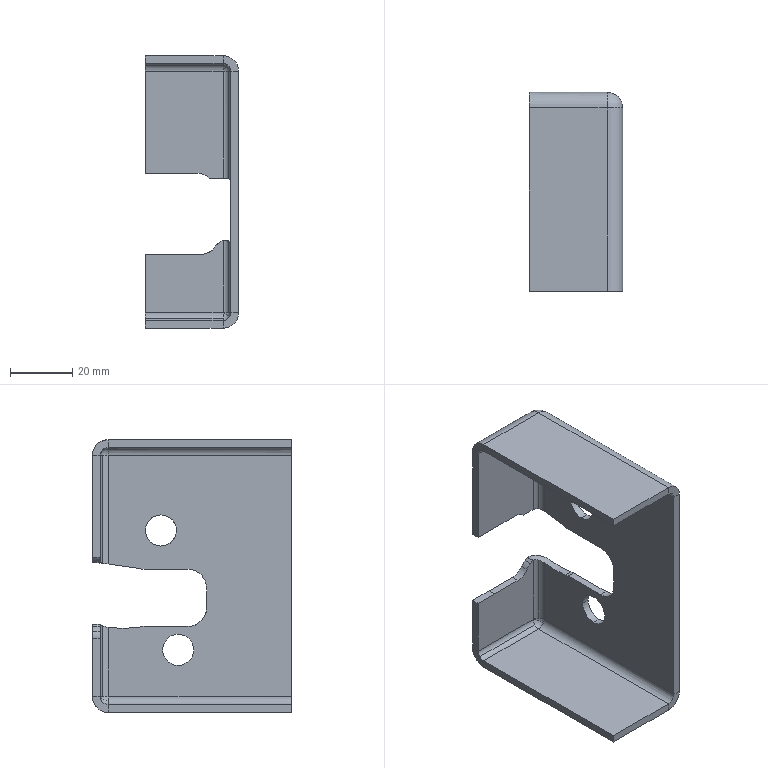Part | NX | features BREP 1 | 1 solid | 75 faces | volume 23694 mm3 | cylinder 32 | plane 30 | sphere 7 | spline 5 | cone 1 | commonest cylinder face diameters 10 x14 5 x11 12 x3 10.001 x1 10.002 x1 10.024 x1